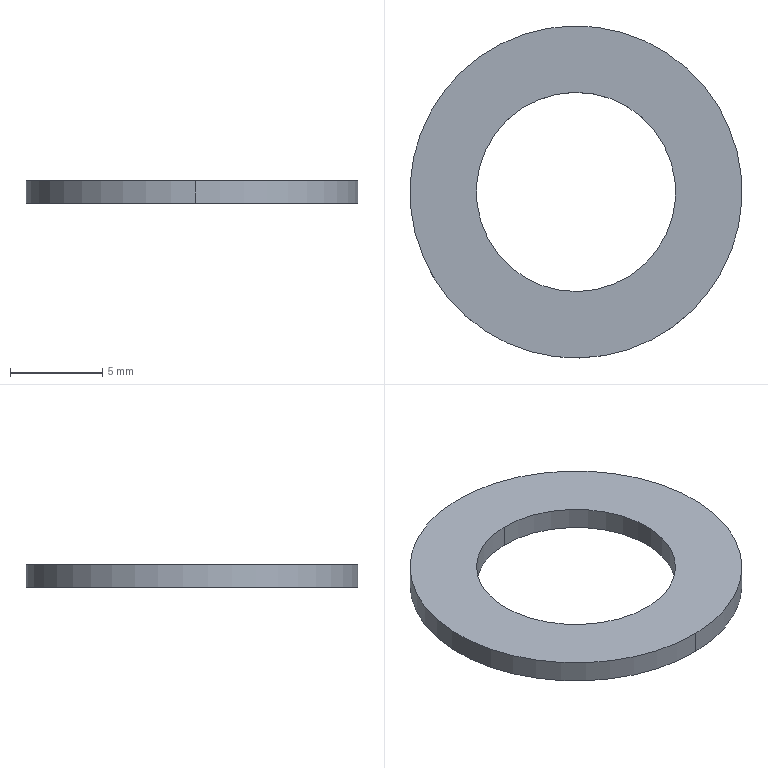Part | SolidWorks | features BaseBody 1 | 1 solid | 6 faces | box 18 x 18 x 1.203 mm | volume 195.432 mm3 | cylinder 4 | plane 2 | commonest cylinder face diameters 10.8 x2 18 x2
STEP:
#1=CARTESIAN_POINT('',(341.658,202.802,1.075));
#2=VERTEX_POINT('',#1);
#3=CARTESIAN_POINT('',(341.885,192.005,1.075));
#4=VERTEX_POINT('',#3);
#5=CARTESIAN_POINT('',(341.771,197.404,1.075));
#6=DIRECTION('',(0.0001435,0.000000521,-1.));
#7=DIRECTION('',(-0.02104,0.9998,-0.000002497));
#8=AXIS2_PLACEMENT_3D('',#5,#6,#7);
#9=CIRCLE('',#8,5.4);
#10=EDGE_CURVE('',#2,#4,#9,.T.);
#11=ORIENTED_EDGE('',*,*,#10,.F.);
#12=CARTESIAN_POINT('',(341.658,202.802,-0.1255));
#13=VERTEX_POINT('',#12);
#14=CARTESIAN_POINT('',(341.658,202.802,1.675));
#15=DIRECTION('',(0.0001435,0.000000521,-1.));
#16=VECTOR('',#15,1000.);
#17=LINE('',#14,#16);
#18=EDGE_CURVE('',#2,#13,#17,.T.);
#19=ORIENTED_EDGE('',*,*,#18,.T.);
#20=CARTESIAN_POINT('',(341.885,192.005,-0.1254));
#21=VERTEX_POINT('',#20);
#22=CARTESIAN_POINT('',(341.772,197.404,-0.1254));
#23=DIRECTION('',(-0.0001435,-0.000000521,1.));
#24=DIRECTION('',(-0.02104,0.9998,-0.000002497));
#25=AXIS2_PLACEMENT_3D('',#22,#23,#24);
#26=CIRCLE('',#25,5.4);
#27=EDGE_CURVE('',#21,#13,#26,.T.);
#28=ORIENTED_EDGE('',*,*,#27,.F.);
#29=CARTESIAN_POINT('',(341.885,192.005,1.675));
#30=DIRECTION('',(0.0001435,0.000000521,-1.));
#31=VECTOR('',#30,1000.);
#32=LINE('',#29,#31);
#33=EDGE_CURVE('',#4,#21,#32,.T.);
#34=ORIENTED_EDGE('',*,*,#33,.F.);
#35=EDGE_LOOP('',(#11,#19,#28,#34));
#36=FACE_OUTER_BOUND('',#35,.T.);
#37=CARTESIAN_POINT('',(341.771,197.404,1.675));
#38=DIRECTION('',(0.0001435,0.000000521,-1.));
#39=DIRECTION('',(0.02104,-0.9998,0.000002497));
#40=AXIS2_PLACEMENT_3D('',#37,#38,#39);
#41=CYLINDRICAL_SURFACE('',#40,5.4);
#42=ADVANCED_FACE('',(#36),#41,.F.);
#43=CARTESIAN_POINT('',(341.582,206.402,1.075));
#44=VERTEX_POINT('',#43);
#45=CARTESIAN_POINT('',(341.961,188.406,1.075));
#46=VERTEX_POINT('',#45);
#47=CARTESIAN_POINT('',(341.771,197.404,1.075));
#48=DIRECTION('',(-0.0001435,-0.000000521,1.));
#49=DIRECTION('',(-0.02104,0.9998,-0.000002497));
#50=AXIS2_PLACEMENT_3D('',#47,#48,#49);
#51=CIRCLE('',#50,9.);
#52=EDGE_CURVE('',#44,#46,#51,.T.);
#53=ORIENTED_EDGE('',*,*,#52,.F.);
#54=CARTESIAN_POINT('',(341.582,206.402,-0.1255));
#55=VERTEX_POINT('',#54);
#56=CARTESIAN_POINT('',(341.582,206.402,1.075));
#57=DIRECTION('',(0.0001435,0.000000521,-1.));
#58=VECTOR('',#57,1000.);
#59=LINE('',#56,#58);
#60=EDGE_CURVE('',#44,#55,#59,.T.);
#61=ORIENTED_EDGE('',*,*,#60,.T.);
#62=CARTESIAN_POINT('',(341.961,188.406,-0.1254));
#63=VERTEX_POINT('',#62);
#64=CARTESIAN_POINT('',(341.772,197.404,-0.1254));
#65=DIRECTION('',(0.0001435,0.000000521,-1.));
#66=DIRECTION('',(-0.02104,0.9998,-0.000002497));
#67=AXIS2_PLACEMENT_3D('',#64,#65,#66);
#68=CIRCLE('',#67,9.);
#69=EDGE_CURVE('',#63,#55,#68,.T.);
#70=ORIENTED_EDGE('',*,*,#69,.F.);
#71=CARTESIAN_POINT('',(341.961,188.406,1.075));
#72=DIRECTION('',(0.0001435,0.000000521,-1.));
#73=VECTOR('',#72,1000.);
#74=LINE('',#71,#73);
#75=EDGE_CURVE('',#46,#63,#74,.T.);
#76=ORIENTED_EDGE('',*,*,#75,.F.);
#77=EDGE_LOOP('',(#53,#61,#70,#76));
#78=FACE_OUTER_BOUND('',#77,.T.);
#79=CARTESIAN_POINT('',(341.771,197.404,1.075));
#80=DIRECTION('',(0.0001435,0.000000521,-1.));
#81=DIRECTION('',(0.02104,-0.9998,0.000002497));
#82=AXIS2_PLACEMENT_3D('',#79,#80,#81);
#83=CYLINDRICAL_SURFACE('',#82,9.);
#84=ADVANCED_FACE('',(#78),#83,.T.);
#85=ORIENTED_EDGE('',*,*,#60,.F.);
#86=CARTESIAN_POINT('',(341.771,197.404,1.075));
#87=DIRECTION('',(-0.0001435,-0.000000521,1.));
#88=DIRECTION('',(-0.02104,0.9998,-0.000002497));
#89=AXIS2_PLACEMENT_3D('',#86,#87,#88);
#90=CIRCLE('',#89,9.);
#91=EDGE_CURVE('',#46,#44,#90,.T.);
#92=ORIENTED_EDGE('',*,*,#91,.F.);
#93=ORIENTED_EDGE('',*,*,#75,.T.);
#94=CARTESIAN_POINT('',(341.772,197.404,-0.1254));
#95=DIRECTION('',(0.0001435,0.000000521,-1.));
#96=DIRECTION('',(-0.02104,0.9998,-0.000002497));
#97=AXIS2_PLACEMENT_3D('',#94,#95,#96);
#98=CIRCLE('',#97,9.);
#99=EDGE_CURVE('',#55,#63,#98,.T.);
#100=ORIENTED_EDGE('',*,*,#99,.F.);
#101=EDGE_LOOP('',(#85,#92,#93,#100));
#102=FACE_OUTER_BOUND('',#101,.T.);
#103=CARTESIAN_POINT('',(341.771,197.404,1.075));
#104=DIRECTION('',(0.0001435,0.000000521,-1.));
#105=DIRECTION('',(0.02104,-0.9998,0.000002497));
#106=AXIS2_PLACEMENT_3D('',#103,#104,#105);
#107=CYLINDRICAL_SURFACE('',#106,9.);
#108=ADVANCED_FACE('',(#102),#107,.T.);
#109=CARTESIAN_POINT('',(341.771,197.404,1.075));
#110=DIRECTION('',(0.0001435,0.000000521,-1.));
#111=DIRECTION('',(-0.02104,0.9998,-0.000002497));
#112=AXIS2_PLACEMENT_3D('',#109,#110,#111);
#113=CIRCLE('',#112,5.4);
#114=EDGE_CURVE('',#4,#2,#113,.T.);
#115=ORIENTED_EDGE('',*,*,#114,.T.);
#116=ORIENTED_EDGE('',*,*,#10,.T.);
#117=EDGE_LOOP('',(#115,#116));
#118=FACE_BOUND('',#117,.T.);
#119=ORIENTED_EDGE('',*,*,#91,.T.);
#120=ORIENTED_EDGE('',*,*,#52,.T.);
#121=EDGE_LOOP('',(#119,#120));
#122=FACE_OUTER_BOUND('',#121,.T.);
#123=CARTESIAN_POINT('',(341.771,197.404,1.075));
#124=DIRECTION('',(-0.0001435,-0.000000521,1.));
#125=DIRECTION('',(-0.003633,1.,0.));
#126=AXIS2_PLACEMENT_3D('',#123,#124,#125);
#127=PLANE('',#126);
#128=ADVANCED_FACE('',(#118,#122),#127,.T.);
#129=ORIENTED_EDGE('',*,*,#18,.F.);
#130=ORIENTED_EDGE('',*,*,#114,.F.);
#131=ORIENTED_EDGE('',*,*,#33,.T.);
#132=CARTESIAN_POINT('',(341.772,197.404,-0.1254));
#133=DIRECTION('',(-0.0001435,-0.000000521,1.));
#134=DIRECTION('',(-0.02104,0.9998,-0.000002497));
#135=AXIS2_PLACEMENT_3D('',#132,#133,#134);
#136=CIRCLE('',#135,5.4);
#137=EDGE_CURVE('',#13,#21,#136,.T.);
#138=ORIENTED_EDGE('',*,*,#137,.F.);
#139=EDGE_LOOP('',(#129,#130,#131,#138));
#140=FACE_OUTER_BOUND('',#139,.T.);
#141=CARTESIAN_POINT('',(341.771,197.404,1.675));
#142=DIRECTION('',(0.0001435,0.000000521,-1.));
#143=DIRECTION('',(0.02104,-0.9998,0.000002497));
#144=AXIS2_PLACEMENT_3D('',#141,#142,#143);
#145=CYLINDRICAL_SURFACE('',#144,5.4);
#146=ADVANCED_FACE('',(#140),#145,.F.);
#147=ORIENTED_EDGE('',*,*,#27,.T.);
#148=ORIENTED_EDGE('',*,*,#137,.T.);
#149=EDGE_LOOP('',(#147,#148));
#150=FACE_BOUND('',#149,.T.);
#151=ORIENTED_EDGE('',*,*,#69,.T.);
#152=ORIENTED_EDGE('',*,*,#99,.T.);
#153=EDGE_LOOP('',(#151,#152));
#154=FACE_OUTER_BOUND('',#153,.T.);
#155=CARTESIAN_POINT('',(341.772,197.404,-0.1254));
#156=DIRECTION('',(0.0001435,0.000000521,-1.));
#157=DIRECTION('',(0.,-1.,-0.000000521));
#158=AXIS2_PLACEMENT_3D('',#155,#156,#157);
#159=PLANE('',#158);
#160=ADVANCED_FACE('',(#150,#154),#159,.T.);
#161=CLOSED_SHELL('',(#42,#84,#108,#128,#146,#160));
#162=MANIFOLD_SOLID_BREP('',#161);
#163=CARTESIAN_POINT('',(0.,0.,0.));
#164=DIRECTION('',(0.,0.,1.));
#165=DIRECTION('',(1.,0.,0.));
#166=AXIS2_PLACEMENT_3D('',#163,#164,#165);
#167=(LENGTH_UNIT()NAMED_UNIT(*)SI_UNIT(.MILLI.,.METRE.));
#168=UNCERTAINTY_MEASURE_WITH_UNIT(LENGTH_MEASURE(0.00001),#167,'','');
#169=(NAMED_UNIT(*)PLANE_ANGLE_UNIT()SI_UNIT($,.RADIAN.));
#170=(NAMED_UNIT(*)SI_UNIT($,.STERADIAN.)SOLID_ANGLE_UNIT());
#171=(GEOMETRIC_REPRESENTATION_CONTEXT(3)GLOBAL_UNCERTAINTY_ASSIGNED_CONTEXT((#168))GLOBAL_UNIT_ASSIGNED_CONTEXT((#167,#169,#170))REPRESENTATION_CONTEXT('',''));
#172=ADVANCED_BREP_SHAPE_REPRESENTATION('',(#162,#166),#171);